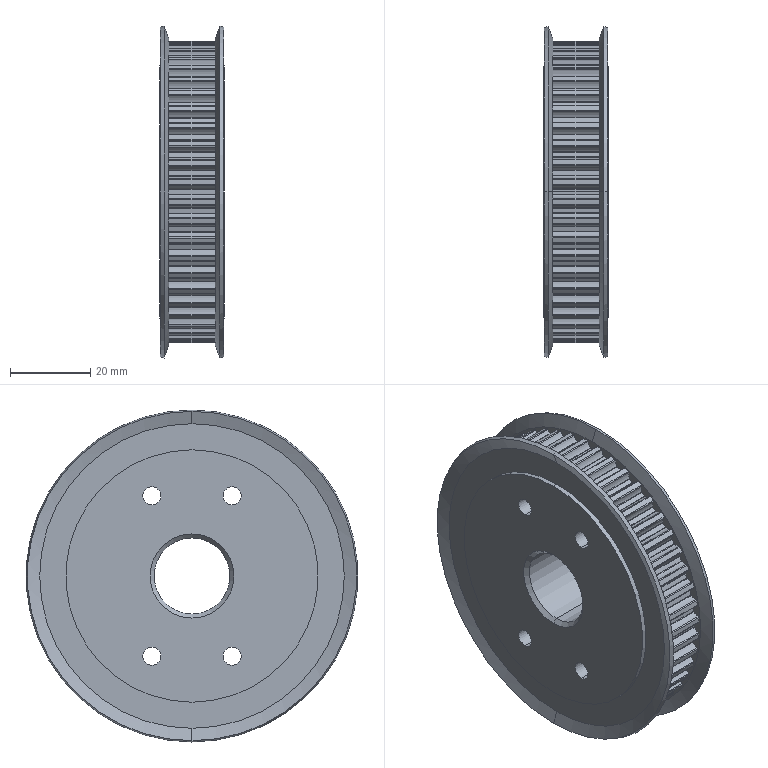Part | SolidWorks | features ICE 2, Chamfer 1, HoleWzd 1, RevCut 1, Revolution 1 | 1 solid | 477 faces | box 16 x 82.872 x 82.872 mm | volume 61065 mm3 | cylinder 451 | cone 16 | plane 10 | commonest cylinder face diameters 0.5 x118 0.4 x110 6.64 x104 71.63 x49 75.25 x48 4.5 x8